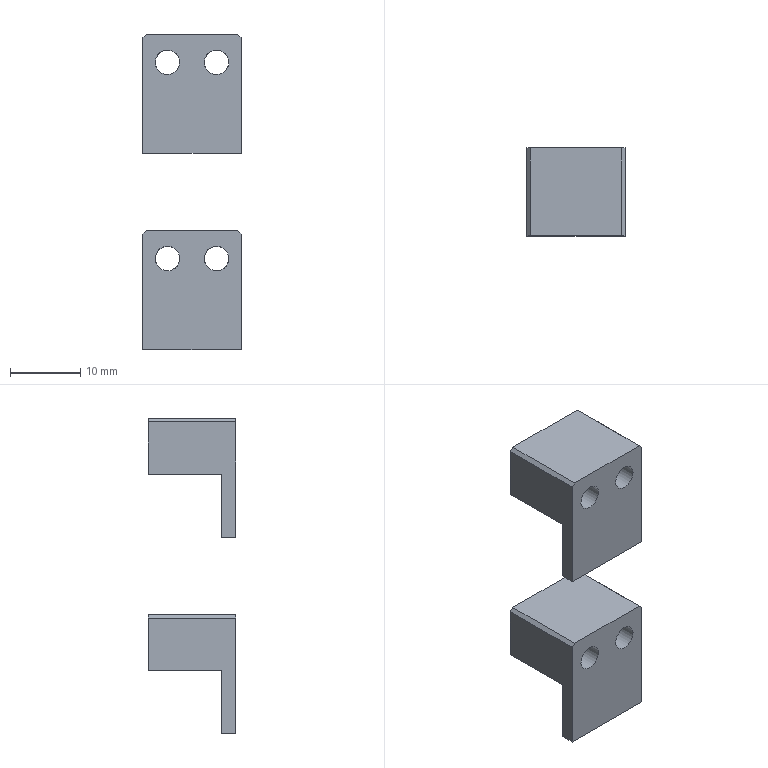CAM job | NX | 3+2 milling, drilling | part box 14 x 12.5 x 45 mm | stock box 15 x 15 x 50 mm
Tools:
number,name,description,diameter,corner_radius,flute_length,length,flutes
9,D10,平底铣刀-粗,10.0,0.0,35.0,75.0,2
7,D6-J,平底铣刀-精,6.0,0.0,25.0,75.0,2
1,D80R0.8飞刀,圆鼻刀-粗,80.0,0.8,50.0,75.0,2
2,D6倒角刀,倒角刀,6.0,0.0,3.0,25.0,2
17,ZT3.5,钻头,3.5,0.0,35.0,50.0,2
Operations:
program,operation,operation_type,tool,method,geometry_group,spindle_rpm,surface_speed,feed_per_tooth,feed_cut,feed_plunge,cut_length_mm,path_length_mm,cut_time_min,machine_time_min
A,顶面,FaceMilling,D80R0.8飞刀,侧刃精光-切深K-步距G,W-A,5000.0,1256.637,0.1,1000.0,100.0,139.0,175.0,0.139,0.1426
A,打点-深0.8,Operation,D6倒角刀,NONE,W-A,8000.0,150.796,0.0312,500.0,90.0,7.2,99.56,0.0144,0.0236
A,通孔-3-4,Operation,ZT3.5,NONE,W-A,3000.0,32.987,0.0333,200.0,90.0,66.206,217.572,0.331,0.3462
A,外形粗_2,VolumeBased25DMillingOperation,D10,METHOD,W-A,8000.0,251.327,0.3125,5000.0,80.0,3367.614,3498.514,0.6735,0.6866
A,底壁粗_1,VolumeBased25DMillingOperation,D10,METHOD,W-A,6000.0,113.0,0.2083,3500.0,100.0,2279.23,2922.467,0.6512,0.7155
A,底精_1,VolumeBased25DMillingOperation,D6-J,METHOD,W-A,6000.0,113.0,0.2083,1200.0,100.0,178.088,328.269,0.1484,0.1634
A,底侧精_3,VolumeBased25DMillingOperation,D6-J,METHOD,W-A,6000.0,113.0,0.2083,1200.0,100.0,94.966,391.978,0.0791,0.1088
A,仅选体,SurfaceContour,D6倒角刀,METHOD,W-A,8000.0,150.796,0.1875,3000.0,100.0,239.31,450.336,0.0798,0.1009
A,DRILL-CHAMFER_1,Operation,D6倒角刀,METHOD,W-A,8000.0,150.796,0.0312,500.0,0.0,20.2,132.792,0.0404,0.0517
A,外形半精_2,VolumeBased25DMillingOperation,D6-J,METHOD,W-A,8000.0,251.327,0.0625,1000.0,100.0,170.36,329.678,0.1704,0.1863